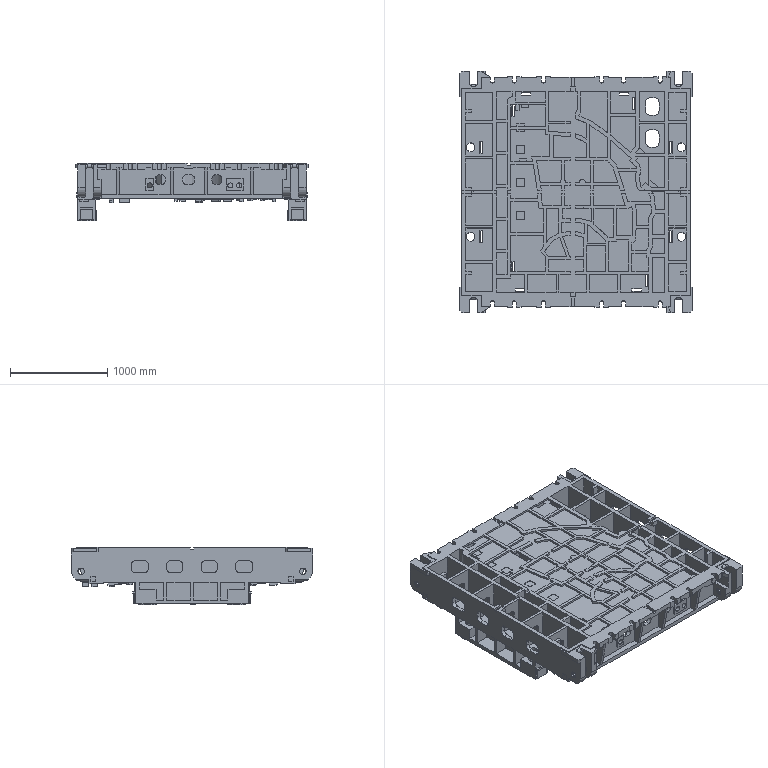Part | NX | features solid 2 | 1 solid | 2454 faces | box 2390 x 2480 x 595 mm | volume 658123198 mm3 | plane 1988 | cylinder 314 | spline 144 | torus 8 | commonest cylinder face diameters 80 x88 68 x48 40 x45 60 x31 20 x24 100 x19